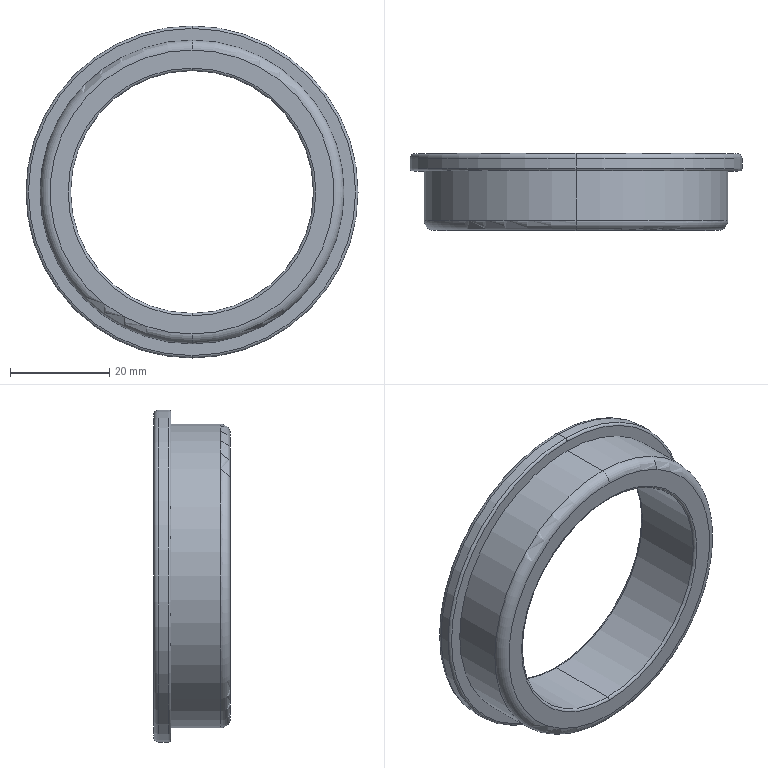Part | SolidWorks | features Fillet 3, ICE 2, Extrusion 1 | 1 solid | 19 faces | box 67 x 15.5 x 67 mm | volume 18291 mm3 | torus 10 | cylinder 6 | plane 3 | commonest cylinder face diameters 49 x2 61.3 x2 67 x2
STEP:
#1=CARTESIAN_POINT('',(0.,0.,-33.));
#2=VERTEX_POINT('',#1);
#3=CARTESIAN_POINT('',(0.,0.,33.));
#4=VERTEX_POINT('',#3);
#5=CARTESIAN_POINT('',(0.,0.,0.));
#6=DIRECTION('',(0.,-1.,0.));
#7=DIRECTION('',(0.,0.,1.));
#8=AXIS2_PLACEMENT_3D('',#5,#6,#7);
#9=CIRCLE('',#8,33.);
#10=EDGE_CURVE('',#2,#4,#9,.T.);
#11=ORIENTED_EDGE('',*,*,#10,.F.);
#12=CARTESIAN_POINT('',(0.,0.5,-33.5));
#13=VERTEX_POINT('',#12);
#14=CARTESIAN_POINT('',(0.,0.5,-33.));
#15=DIRECTION('',(1.,0.,0.));
#16=DIRECTION('',(0.,0.,-1.));
#17=AXIS2_PLACEMENT_3D('',#14,#15,#16);
#18=CIRCLE('',#17,0.5);
#19=EDGE_CURVE('',#2,#13,#18,.T.);
#20=ORIENTED_EDGE('',*,*,#19,.T.);
#21=CARTESIAN_POINT('',(0.,0.5,33.5));
#22=VERTEX_POINT('',#21);
#23=CARTESIAN_POINT('',(0.,0.5,0.));
#24=DIRECTION('',(0.,1.,0.));
#25=DIRECTION('',(0.,0.,1.));
#26=AXIS2_PLACEMENT_3D('',#23,#24,#25);
#27=CIRCLE('',#26,33.5);
#28=EDGE_CURVE('',#22,#13,#27,.T.);
#29=ORIENTED_EDGE('',*,*,#28,.F.);
#30=CARTESIAN_POINT('',(0.,0.5,33.));
#31=DIRECTION('',(-1.,0.,0.));
#32=DIRECTION('',(0.,0.,1.));
#33=AXIS2_PLACEMENT_3D('',#30,#31,#32);
#34=CIRCLE('',#33,0.5);
#35=EDGE_CURVE('',#4,#22,#34,.T.);
#36=ORIENTED_EDGE('',*,*,#35,.F.);
#37=EDGE_LOOP('',(#11,#20,#29,#36));
#38=FACE_OUTER_BOUND('',#37,.T.);
#39=CARTESIAN_POINT('',(0.,0.5,0.));
#40=DIRECTION('',(0.,1.,0.));
#41=DIRECTION('',(0.,0.,1.));
#42=AXIS2_PLACEMENT_3D('',#39,#40,#41);
#43=TOROIDAL_SURFACE('',#42,33.,0.5);
#44=ADVANCED_FACE('',(#38),#43,.T.);
#45=CARTESIAN_POINT('',(0.,-11.5,-24.5));
#46=VERTEX_POINT('',#45);
#47=CARTESIAN_POINT('',(0.,-11.5,24.5));
#48=VERTEX_POINT('',#47);
#49=CARTESIAN_POINT('',(0.,-11.5,0.));
#50=DIRECTION('',(0.,-1.,0.));
#51=DIRECTION('',(0.,0.,1.));
#52=AXIS2_PLACEMENT_3D('',#49,#50,#51);
#53=CIRCLE('',#52,24.5);
#54=EDGE_CURVE('',#46,#48,#53,.T.);
#55=ORIENTED_EDGE('',*,*,#54,.F.);
#56=CARTESIAN_POINT('',(0.,-12.,-25.));
#57=VERTEX_POINT('',#56);
#58=CARTESIAN_POINT('',(0.,-11.5,-25.));
#59=DIRECTION('',(1.,0.,0.));
#60=DIRECTION('',(0.,0.,-1.));
#61=AXIS2_PLACEMENT_3D('',#58,#59,#60);
#62=CIRCLE('',#61,0.5);
#63=EDGE_CURVE('',#46,#57,#62,.T.);
#64=ORIENTED_EDGE('',*,*,#63,.T.);
#65=CARTESIAN_POINT('',(0.,-12.,25.));
#66=VERTEX_POINT('',#65);
#67=CARTESIAN_POINT('',(0.,-12.,0.));
#68=DIRECTION('',(0.,1.,0.));
#69=DIRECTION('',(0.,0.,1.));
#70=AXIS2_PLACEMENT_3D('',#67,#68,#69);
#71=CIRCLE('',#70,25.);
#72=EDGE_CURVE('',#66,#57,#71,.T.);
#73=ORIENTED_EDGE('',*,*,#72,.F.);
#74=CARTESIAN_POINT('',(0.,-11.5,25.));
#75=DIRECTION('',(-1.,0.,0.));
#76=DIRECTION('',(0.,0.,1.));
#77=AXIS2_PLACEMENT_3D('',#74,#75,#76);
#78=CIRCLE('',#77,0.5);
#79=EDGE_CURVE('',#48,#66,#78,.T.);
#80=ORIENTED_EDGE('',*,*,#79,.F.);
#81=EDGE_LOOP('',(#55,#64,#73,#80));
#82=FACE_OUTER_BOUND('',#81,.T.);
#83=CARTESIAN_POINT('',(0.,-11.5,0.));
#84=DIRECTION('',(0.,1.,0.));
#85=DIRECTION('',(0.,0.,1.));
#86=AXIS2_PLACEMENT_3D('',#83,#84,#85);
#87=TOROIDAL_SURFACE('',#86,25.,0.5);
#88=ADVANCED_FACE('',(#82),#87,.T.);
#89=CARTESIAN_POINT('',(0.,3.5,-25.));
#90=VERTEX_POINT('',#89);
#91=CARTESIAN_POINT('',(0.,3.5,25.));
#92=VERTEX_POINT('',#91);
#93=CARTESIAN_POINT('',(0.,3.5,0.));
#94=DIRECTION('',(0.,-1.,0.));
#95=DIRECTION('',(0.,0.,1.));
#96=AXIS2_PLACEMENT_3D('',#93,#94,#95);
#97=CIRCLE('',#96,25.);
#98=EDGE_CURVE('',#90,#92,#97,.T.);
#99=ORIENTED_EDGE('',*,*,#98,.F.);
#100=CARTESIAN_POINT('',(0.,3.,-24.5));
#101=VERTEX_POINT('',#100);
#102=CARTESIAN_POINT('',(0.,3.,-25.));
#103=DIRECTION('',(1.,0.,0.));
#104=DIRECTION('',(0.,0.,-1.));
#105=AXIS2_PLACEMENT_3D('',#102,#103,#104);
#106=CIRCLE('',#105,0.5);
#107=EDGE_CURVE('',#90,#101,#106,.T.);
#108=ORIENTED_EDGE('',*,*,#107,.T.);
#109=CARTESIAN_POINT('',(0.,3.,24.5));
#110=VERTEX_POINT('',#109);
#111=CARTESIAN_POINT('',(0.,3.,0.));
#112=DIRECTION('',(0.,1.,0.));
#113=DIRECTION('',(0.,0.,1.));
#114=AXIS2_PLACEMENT_3D('',#111,#112,#113);
#115=CIRCLE('',#114,24.5);
#116=EDGE_CURVE('',#110,#101,#115,.T.);
#117=ORIENTED_EDGE('',*,*,#116,.F.);
#118=CARTESIAN_POINT('',(0.,3.,25.));
#119=DIRECTION('',(-1.,0.,0.));
#120=DIRECTION('',(0.,0.,1.));
#121=AXIS2_PLACEMENT_3D('',#118,#119,#120);
#122=CIRCLE('',#121,0.5);
#123=EDGE_CURVE('',#92,#110,#122,.T.);
#124=ORIENTED_EDGE('',*,*,#123,.F.);
#125=EDGE_LOOP('',(#99,#108,#117,#124));
#126=FACE_OUTER_BOUND('',#125,.T.);
#127=CARTESIAN_POINT('',(0.,3.,0.));
#128=DIRECTION('',(0.,1.,0.));
#129=DIRECTION('',(0.,0.,1.));
#130=AXIS2_PLACEMENT_3D('',#127,#128,#129);
#131=TOROIDAL_SURFACE('',#130,25.,0.5);
#132=ADVANCED_FACE('',(#126),#131,.T.);
#133=CARTESIAN_POINT('',(0.,-12.,-28.65));
#134=VERTEX_POINT('',#133);
#135=CARTESIAN_POINT('',(0.,-12.,28.65));
#136=VERTEX_POINT('',#135);
#137=CARTESIAN_POINT('',(0.,-12.,0.));
#138=DIRECTION('',(0.,-1.,0.));
#139=DIRECTION('',(0.,0.,1.));
#140=AXIS2_PLACEMENT_3D('',#137,#138,#139);
#141=CIRCLE('',#140,28.65);
#142=EDGE_CURVE('',#134,#136,#141,.T.);
#143=ORIENTED_EDGE('',*,*,#142,.F.);
#144=CARTESIAN_POINT('',(0.,-10.,-30.65));
#145=VERTEX_POINT('',#144);
#146=CARTESIAN_POINT('',(0.,-10.,-28.65));
#147=DIRECTION('',(1.,0.,0.));
#148=DIRECTION('',(0.,0.,-1.));
#149=AXIS2_PLACEMENT_3D('',#146,#147,#148);
#150=CIRCLE('',#149,2.);
#151=EDGE_CURVE('',#134,#145,#150,.T.);
#152=ORIENTED_EDGE('',*,*,#151,.T.);
#153=CARTESIAN_POINT('',(0.,-10.,30.65));
#154=VERTEX_POINT('',#153);
#155=CARTESIAN_POINT('',(0.,-10.,0.));
#156=DIRECTION('',(0.,1.,0.));
#157=DIRECTION('',(0.,0.,1.));
#158=AXIS2_PLACEMENT_3D('',#155,#156,#157);
#159=CIRCLE('',#158,30.65);
#160=EDGE_CURVE('',#154,#145,#159,.T.);
#161=ORIENTED_EDGE('',*,*,#160,.F.);
#162=CARTESIAN_POINT('',(0.,-10.,28.65));
#163=DIRECTION('',(-1.,0.,0.));
#164=DIRECTION('',(0.,0.,1.));
#165=AXIS2_PLACEMENT_3D('',#162,#163,#164);
#166=CIRCLE('',#165,2.);
#167=EDGE_CURVE('',#136,#154,#166,.T.);
#168=ORIENTED_EDGE('',*,*,#167,.F.);
#169=EDGE_LOOP('',(#143,#152,#161,#168));
#170=FACE_OUTER_BOUND('',#169,.T.);
#171=CARTESIAN_POINT('',(0.,-10.,0.));
#172=DIRECTION('',(0.,1.,0.));
#173=DIRECTION('',(0.,0.,1.));
#174=AXIS2_PLACEMENT_3D('',#171,#172,#173);
#175=TOROIDAL_SURFACE('',#174,28.65,2.);
#176=ADVANCED_FACE('',(#170),#175,.T.);
#177=CARTESIAN_POINT('',(0.,2.5,-33.5));
#178=VERTEX_POINT('',#177);
#179=CARTESIAN_POINT('',(0.,2.5,33.5));
#180=VERTEX_POINT('',#179);
#181=CARTESIAN_POINT('',(0.,2.5,0.));
#182=DIRECTION('',(0.,-1.,0.));
#183=DIRECTION('',(0.,0.,1.));
#184=AXIS2_PLACEMENT_3D('',#181,#182,#183);
#185=CIRCLE('',#184,33.5);
#186=EDGE_CURVE('',#178,#180,#185,.T.);
#187=ORIENTED_EDGE('',*,*,#186,.F.);
#188=CARTESIAN_POINT('',(0.,3.5,-32.5));
#189=VERTEX_POINT('',#188);
#190=CARTESIAN_POINT('',(0.,2.5,-32.5));
#191=DIRECTION('',(1.,0.,0.));
#192=DIRECTION('',(0.,0.,-1.));
#193=AXIS2_PLACEMENT_3D('',#190,#191,#192);
#194=CIRCLE('',#193,1.);
#195=EDGE_CURVE('',#178,#189,#194,.T.);
#196=ORIENTED_EDGE('',*,*,#195,.T.);
#197=CARTESIAN_POINT('',(0.,3.5,32.5));
#198=VERTEX_POINT('',#197);
#199=CARTESIAN_POINT('',(0.,3.5,0.));
#200=DIRECTION('',(0.,1.,0.));
#201=DIRECTION('',(0.,0.,1.));
#202=AXIS2_PLACEMENT_3D('',#199,#200,#201);
#203=CIRCLE('',#202,32.5);
#204=EDGE_CURVE('',#198,#189,#203,.T.);
#205=ORIENTED_EDGE('',*,*,#204,.F.);
#206=CARTESIAN_POINT('',(0.,2.5,32.5));
#207=DIRECTION('',(-1.,0.,0.));
#208=DIRECTION('',(0.,0.,1.));
#209=AXIS2_PLACEMENT_3D('',#206,#207,#208);
#210=CIRCLE('',#209,1.);
#211=EDGE_CURVE('',#180,#198,#210,.T.);
#212=ORIENTED_EDGE('',*,*,#211,.F.);
#213=EDGE_LOOP('',(#187,#196,#205,#212));
#214=FACE_OUTER_BOUND('',#213,.T.);
#215=CARTESIAN_POINT('',(0.,2.5,0.));
#216=DIRECTION('',(0.,1.,0.));
#217=DIRECTION('',(0.,0.,1.));
#218=AXIS2_PLACEMENT_3D('',#215,#216,#217);
#219=TOROIDAL_SURFACE('',#218,32.5,1.);
#220=ADVANCED_FACE('',(#214),#219,.T.);
#221=CARTESIAN_POINT('',(0.,-11.5,0.));
#222=DIRECTION('',(0.,-1.,0.));
#223=DIRECTION('',(0.,0.,1.));
#224=AXIS2_PLACEMENT_3D('',#221,#222,#223);
#225=CIRCLE('',#224,24.5);
#226=EDGE_CURVE('',#48,#46,#225,.T.);
#227=ORIENTED_EDGE('',*,*,#226,.T.);
#228=CARTESIAN_POINT('',(0.,-12.,-24.5));
#229=DIRECTION('',(0.,1.,0.));
#230=VECTOR('',#229,1000.);
#231=LINE('',#228,#230);
#232=EDGE_CURVE('',#46,#101,#231,.T.);
#233=ORIENTED_EDGE('',*,*,#232,.T.);
#234=CARTESIAN_POINT('',(0.,3.,0.));
#235=DIRECTION('',(0.,1.,0.));
#236=DIRECTION('',(0.,0.,1.));
#237=AXIS2_PLACEMENT_3D('',#234,#235,#236);
#238=CIRCLE('',#237,24.5);
#239=EDGE_CURVE('',#101,#110,#238,.T.);
#240=ORIENTED_EDGE('',*,*,#239,.T.);
#241=CARTESIAN_POINT('',(0.,-12.,24.5));
#242=DIRECTION('',(0.,1.,0.));
#243=VECTOR('',#242,1000.);
#244=LINE('',#241,#243);
#245=EDGE_CURVE('',#48,#110,#244,.T.);
#246=ORIENTED_EDGE('',*,*,#245,.F.);
#247=EDGE_LOOP('',(#227,#233,#240,#246));
#248=FACE_OUTER_BOUND('',#247,.T.);
#249=CARTESIAN_POINT('',(0.,-12.,0.));
#250=DIRECTION('',(0.,1.,0.));
#251=DIRECTION('',(0.,0.,1.));
#252=AXIS2_PLACEMENT_3D('',#249,#250,#251);
#253=CYLINDRICAL_SURFACE('',#252,24.5);
#254=ADVANCED_FACE('',(#248),#253,.F.);
#255=ORIENTED_EDGE('',*,*,#186,.T.);
#256=CARTESIAN_POINT('',(0.,3.5,33.5));
#257=DIRECTION('',(0.,-1.,0.));
#258=VECTOR('',#257,1000.);
#259=LINE('',#256,#258);
#260=EDGE_CURVE('',#180,#22,#259,.T.);
#261=ORIENTED_EDGE('',*,*,#260,.T.);
#262=ORIENTED_EDGE('',*,*,#28,.T.);
#263=CARTESIAN_POINT('',(0.,3.5,-33.5));
#264=DIRECTION('',(0.,-1.,0.));
#265=VECTOR('',#264,1000.);
#266=LINE('',#263,#265);
#267=EDGE_CURVE('',#178,#13,#266,.T.);
#268=ORIENTED_EDGE('',*,*,#267,.F.);
#269=EDGE_LOOP('',(#255,#261,#262,#268));
#270=FACE_OUTER_BOUND('',#269,.T.);
#271=CARTESIAN_POINT('',(0.,3.5,0.));
#272=DIRECTION('',(0.,-1.,0.));
#273=DIRECTION('',(0.,0.,-1.));
#274=AXIS2_PLACEMENT_3D('',#271,#272,#273);
#275=CYLINDRICAL_SURFACE('',#274,33.5);
#276=ADVANCED_FACE('',(#270),#275,.T.);
#277=ORIENTED_EDGE('',*,*,#160,.T.);
#278=CARTESIAN_POINT('',(0.,0.,-30.65));
#279=VERTEX_POINT('',#278);
#280=CARTESIAN_POINT('',(0.,-12.,-30.65));
#281=DIRECTION('',(0.,1.,0.));
#282=VECTOR('',#281,1000.);
#283=LINE('',#280,#282);
#284=EDGE_CURVE('',#145,#279,#283,.T.);
#285=ORIENTED_EDGE('',*,*,#284,.T.);
#286=CARTESIAN_POINT('',(0.,0.,30.65));
#287=VERTEX_POINT('',#286);
#288=CARTESIAN_POINT('',(0.,0.,0.));
#289=DIRECTION('',(0.,1.,0.));
#290=DIRECTION('',(0.,0.,1.));
#291=AXIS2_PLACEMENT_3D('',#288,#289,#290);
#292=CIRCLE('',#291,30.65);
#293=EDGE_CURVE('',#287,#279,#292,.T.);
#294=ORIENTED_EDGE('',*,*,#293,.F.);
#295=CARTESIAN_POINT('',(0.,-12.,30.65));
#296=DIRECTION('',(0.,1.,0.));
#297=VECTOR('',#296,1000.);
#298=LINE('',#295,#297);
#299=EDGE_CURVE('',#154,#287,#298,.T.);
#300=ORIENTED_EDGE('',*,*,#299,.F.);
#301=EDGE_LOOP('',(#277,#285,#294,#300));
#302=FACE_OUTER_BOUND('',#301,.T.);
#303=CARTESIAN_POINT('',(0.,-12.,0.));
#304=DIRECTION('',(0.,1.,0.));
#305=DIRECTION('',(0.,0.,1.));
#306=AXIS2_PLACEMENT_3D('',#303,#304,#305);
#307=CYLINDRICAL_SURFACE('',#306,30.65);
#308=ADVANCED_FACE('',(#302),#307,.T.);
#309=ORIENTED_EDGE('',*,*,#284,.F.);
#310=CARTESIAN_POINT('',(0.,-10.,0.));
#311=DIRECTION('',(0.,1.,0.));
#312=DIRECTION('',(0.,0.,1.));
#313=AXIS2_PLACEMENT_3D('',#310,#311,#312);
#314=CIRCLE('',#313,30.65);
#315=EDGE_CURVE('',#145,#154,#314,.T.);
#316=ORIENTED_EDGE('',*,*,#315,.T.);
#317=ORIENTED_EDGE('',*,*,#299,.T.);
#318=CARTESIAN_POINT('',(0.,0.,0.));
#319=DIRECTION('',(0.,1.,0.));
#320=DIRECTION('',(0.,0.,1.));
#321=AXIS2_PLACEMENT_3D('',#318,#319,#320);
#322=CIRCLE('',#321,30.65);
#323=EDGE_CURVE('',#279,#287,#322,.T.);
#324=ORIENTED_EDGE('',*,*,#323,.F.);
#325=EDGE_LOOP('',(#309,#316,#317,#324));
#326=FACE_OUTER_BOUND('',#325,.T.);
#327=CARTESIAN_POINT('',(0.,-12.,0.));
#328=DIRECTION('',(0.,1.,0.));
#329=DIRECTION('',(0.,0.,1.));
#330=AXIS2_PLACEMENT_3D('',#327,#328,#329);
#331=CYLINDRICAL_SURFACE('',#330,30.65);
#332=ADVANCED_FACE('',(#326),#331,.T.);
#333=ORIENTED_EDGE('',*,*,#72,.T.);
#334=CARTESIAN_POINT('',(0.,-12.,0.));
#335=DIRECTION('',(0.,1.,0.));
#336=DIRECTION('',(0.,0.,1.));
#337=AXIS2_PLACEMENT_3D('',#334,#335,#336);
#338=CIRCLE('',#337,25.);
#339=EDGE_CURVE('',#57,#66,#338,.T.);
#340=ORIENTED_EDGE('',*,*,#339,.T.);
#341=EDGE_LOOP('',(#333,#340));
#342=FACE_BOUND('',#341,.T.);
#343=CARTESIAN_POINT('',(0.,-12.,0.));
#344=DIRECTION('',(0.,-1.,0.));
#345=DIRECTION('',(0.,0.,1.));
#346=AXIS2_PLACEMENT_3D('',#343,#344,#345);
#347=CIRCLE('',#346,28.65);
#348=EDGE_CURVE('',#136,#134,#347,.T.);
#349=ORIENTED_EDGE('',*,*,#348,.T.);
#350=ORIENTED_EDGE('',*,*,#142,.T.);
#351=EDGE_LOOP('',(#349,#350));
#352=FACE_OUTER_BOUND('',#351,.T.);
#353=CARTESIAN_POINT('',(0.,-12.,0.));
#354=DIRECTION('',(0.,1.,0.));
#355=DIRECTION('',(0.,0.,1.));
#356=AXIS2_PLACEMENT_3D('',#353,#354,#355);
#357=PLANE('',#356);
#358=ADVANCED_FACE('',(#342,#352),#357,.F.);
#359=ORIENTED_EDGE('',*,*,#260,.F.);
#360=CARTESIAN_POINT('',(0.,2.5,0.));
#361=DIRECTION('',(0.,-1.,0.));
#362=DIRECTION('',(0.,0.,1.));
#363=AXIS2_PLACEMENT_3D('',#360,#361,#362);
#364=CIRCLE('',#363,33.5);
#365=EDGE_CURVE('',#180,#178,#364,.T.);
#366=ORIENTED_EDGE('',*,*,#365,.T.);
#367=ORIENTED_EDGE('',*,*,#267,.T.);
#368=CARTESIAN_POINT('',(0.,0.5,0.));
#369=DIRECTION('',(0.,1.,0.));
#370=DIRECTION('',(0.,0.,1.));
#371=AXIS2_PLACEMENT_3D('',#368,#369,#370);
#372=CIRCLE('',#371,33.5);
#373=EDGE_CURVE('',#13,#22,#372,.T.);
#374=ORIENTED_EDGE('',*,*,#373,.T.);
#375=EDGE_LOOP('',(#359,#366,#367,#374));
#376=FACE_OUTER_BOUND('',#375,.T.);
#377=CARTESIAN_POINT('',(0.,3.5,0.));
#378=DIRECTION('',(0.,-1.,0.));
#379=DIRECTION('',(0.,0.,-1.));
#380=AXIS2_PLACEMENT_3D('',#377,#378,#379);
#381=CYLINDRICAL_SURFACE('',#380,33.5);
#382=ADVANCED_FACE('',(#376),#381,.T.);
#383=CARTESIAN_POINT('',(0.,3.5,0.));
#384=DIRECTION('',(0.,-1.,0.));
#385=DIRECTION('',(0.,0.,1.));
#386=AXIS2_PLACEMENT_3D('',#383,#384,#385);
#387=CIRCLE('',#386,25.);
#388=EDGE_CURVE('',#92,#90,#387,.T.);
#389=ORIENTED_EDGE('',*,*,#388,.T.);
#390=ORIENTED_EDGE('',*,*,#98,.T.);
#391=EDGE_LOOP('',(#389,#390));
#392=FACE_BOUND('',#391,.T.);
#393=ORIENTED_EDGE('',*,*,#204,.T.);
#394=CARTESIAN_POINT('',(0.,3.5,0.));
#395=DIRECTION('',(0.,1.,0.));
#396=DIRECTION('',(0.,0.,1.));
#397=AXIS2_PLACEMENT_3D('',#394,#395,#396);
#398=CIRCLE('',#397,32.5);
#399=EDGE_CURVE('',#189,#198,#398,.T.);
#400=ORIENTED_EDGE('',*,*,#399,.T.);
#401=EDGE_LOOP('',(#393,#400));
#402=FACE_OUTER_BOUND('',#401,.T.);
#403=CARTESIAN_POINT('',(0.,3.5,0.));
#404=DIRECTION('',(0.,1.,0.));
#405=DIRECTION('',(0.,0.,1.));
#406=AXIS2_PLACEMENT_3D('',#403,#404,#405);
#407=PLANE('',#406);
#408=ADVANCED_FACE('',(#392,#402),#407,.T.);
#409=CARTESIAN_POINT('',(0.,0.,0.));
#410=DIRECTION('',(0.,-1.,0.));
#411=DIRECTION('',(0.,0.,1.));
#412=AXIS2_PLACEMENT_3D('',#409,#410,#411);
#413=CIRCLE('',#412,33.);
#414=EDGE_CURVE('',#4,#2,#413,.T.);
#415=ORIENTED_EDGE('',*,*,#414,.T.);
#416=ORIENTED_EDGE('',*,*,#10,.T.);
#417=EDGE_LOOP('',(#415,#416));
#418=FACE_OUTER_BOUND('',#417,.T.);
#419=ORIENTED_EDGE('',*,*,#293,.T.);
#420=ORIENTED_EDGE('',*,*,#323,.T.);
#421=EDGE_LOOP('',(#419,#420));
#422=FACE_BOUND('',#421,.T.);
#423=CARTESIAN_POINT('',(0.,0.,0.));
#424=DIRECTION('',(0.,1.,0.));
#425=DIRECTION('',(0.,0.,1.));
#426=AXIS2_PLACEMENT_3D('',#423,#424,#425);
#427=PLANE('',#426);
#428=ADVANCED_FACE('',(#418,#422),#427,.F.);
#429=ORIENTED_EDGE('',*,*,#232,.F.);
#430=ORIENTED_EDGE('',*,*,#54,.T.);
#431=ORIENTED_EDGE('',*,*,#245,.T.);
#432=ORIENTED_EDGE('',*,*,#116,.T.);
#433=EDGE_LOOP('',(#429,#430,#431,#432));
#434=FACE_OUTER_BOUND('',#433,.T.);
#435=CARTESIAN_POINT('',(0.,-12.,0.));
#436=DIRECTION('',(0.,1.,0.));
#437=DIRECTION('',(0.,0.,1.));
#438=AXIS2_PLACEMENT_3D('',#435,#436,#437);
#439=CYLINDRICAL_SURFACE('',#438,24.5);
#440=ADVANCED_FACE('',(#434),#439,.F.);
#441=ORIENTED_EDGE('',*,*,#195,.F.);
#442=ORIENTED_EDGE('',*,*,#365,.F.);
#443=ORIENTED_EDGE('',*,*,#211,.T.);
#444=ORIENTED_EDGE('',*,*,#399,.F.);
#445=EDGE_LOOP('',(#441,#442,#443,#444));
#446=FACE_OUTER_BOUND('',#445,.T.);
#447=CARTESIAN_POINT('',(0.,2.5,0.));
#448=DIRECTION('',(0.,1.,0.));
#449=DIRECTION('',(0.,0.,1.));
#450=AXIS2_PLACEMENT_3D('',#447,#448,#449);
#451=TOROIDAL_SURFACE('',#450,32.5,1.);
#452=ADVANCED_FACE('',(#446),#451,.T.);
#453=ORIENTED_EDGE('',*,*,#151,.F.);
#454=ORIENTED_EDGE('',*,*,#348,.F.);
#455=ORIENTED_EDGE('',*,*,#167,.T.);
#456=ORIENTED_EDGE('',*,*,#315,.F.);
#457=EDGE_LOOP('',(#453,#454,#455,#456));
#458=FACE_OUTER_BOUND('',#457,.T.);
#459=CARTESIAN_POINT('',(0.,-10.,0.));
#460=DIRECTION('',(0.,1.,0.));
#461=DIRECTION('',(0.,0.,1.));
#462=AXIS2_PLACEMENT_3D('',#459,#460,#461);
#463=TOROIDAL_SURFACE('',#462,28.65,2.);
#464=ADVANCED_FACE('',(#458),#463,.T.);
#465=ORIENTED_EDGE('',*,*,#107,.F.);
#466=ORIENTED_EDGE('',*,*,#388,.F.);
#467=ORIENTED_EDGE('',*,*,#123,.T.);
#468=ORIENTED_EDGE('',*,*,#239,.F.);
#469=EDGE_LOOP('',(#465,#466,#467,#468));
#470=FACE_OUTER_BOUND('',#469,.T.);
#471=CARTESIAN_POINT('',(0.,3.,0.));
#472=DIRECTION('',(0.,1.,0.));
#473=DIRECTION('',(0.,0.,1.));
#474=AXIS2_PLACEMENT_3D('',#471,#472,#473);
#475=TOROIDAL_SURFACE('',#474,25.,0.5);
#476=ADVANCED_FACE('',(#470),#475,.T.);
#477=ORIENTED_EDGE('',*,*,#63,.F.);
#478=ORIENTED_EDGE('',*,*,#226,.F.);
#479=ORIENTED_EDGE('',*,*,#79,.T.);
#480=ORIENTED_EDGE('',*,*,#339,.F.);
#481=EDGE_LOOP('',(#477,#478,#479,#480));
#482=FACE_OUTER_BOUND('',#481,.T.);
#483=CARTESIAN_POINT('',(0.,-11.5,0.));
#484=DIRECTION('',(0.,1.,0.));
#485=DIRECTION('',(0.,0.,1.));
#486=AXIS2_PLACEMENT_3D('',#483,#484,#485);
#487=TOROIDAL_SURFACE('',#486,25.,0.5);
#488=ADVANCED_FACE('',(#482),#487,.T.);
#489=ORIENTED_EDGE('',*,*,#19,.F.);
#490=ORIENTED_EDGE('',*,*,#414,.F.);
#491=ORIENTED_EDGE('',*,*,#35,.T.);
#492=ORIENTED_EDGE('',*,*,#373,.F.);
#493=EDGE_LOOP('',(#489,#490,#491,#492));
#494=FACE_OUTER_BOUND('',#493,.T.);
#495=CARTESIAN_POINT('',(0.,0.5,0.));
#496=DIRECTION('',(0.,1.,0.));
#497=DIRECTION('',(0.,0.,1.));
#498=AXIS2_PLACEMENT_3D('',#495,#496,#497);
#499=TOROIDAL_SURFACE('',#498,33.,0.5);
#500=ADVANCED_FACE('',(#494),#499,.T.);
#501=CLOSED_SHELL('',(#44,#88,#132,#176,#220,#254,#276,#308,#332,#358,#382,#408,#428,#440,#452,#464,#476,#488,#500));
#502=MANIFOLD_SOLID_BREP('',#501);
#503=CARTESIAN_POINT('',(0.,0.,0.));
#504=DIRECTION('',(0.,0.,1.));
#505=DIRECTION('',(1.,0.,0.));
#506=AXIS2_PLACEMENT_3D('',#503,#504,#505);
#507=(LENGTH_UNIT()NAMED_UNIT(*)SI_UNIT(.MILLI.,.METRE.));
#508=UNCERTAINTY_MEASURE_WITH_UNIT(LENGTH_MEASURE(0.00001),#507,'','');
#509=(NAMED_UNIT(*)PLANE_ANGLE_UNIT()SI_UNIT($,.RADIAN.));
#510=(NAMED_UNIT(*)SI_UNIT($,.STERADIAN.)SOLID_ANGLE_UNIT());
#511=(GEOMETRIC_REPRESENTATION_CONTEXT(3)GLOBAL_UNCERTAINTY_ASSIGNED_CONTEXT((#508))GLOBAL_UNIT_ASSIGNED_CONTEXT((#507,#509,#510))REPRESENTATION_CONTEXT('',''));
#512=ADVANCED_BREP_SHAPE_REPRESENTATION('',(#502,#506),#511);